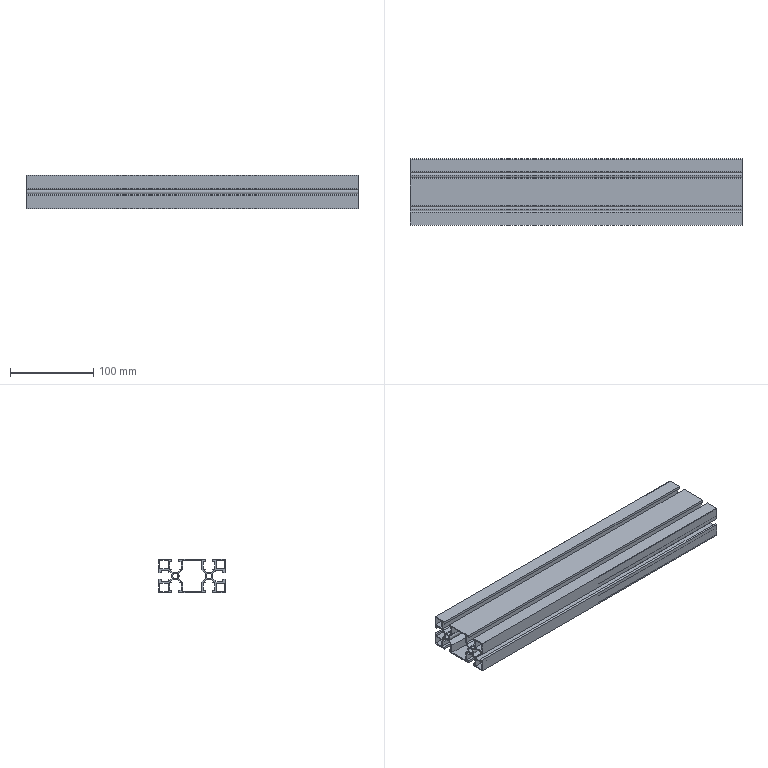Part | 1 solid | 126 faces | box 400 x 80 x 40 mm | volume 277435 mm3 | plane 110 | cylinder 16 | commonest cylinder face diameters 9.6 x10 6.6 x4 0.6 x2